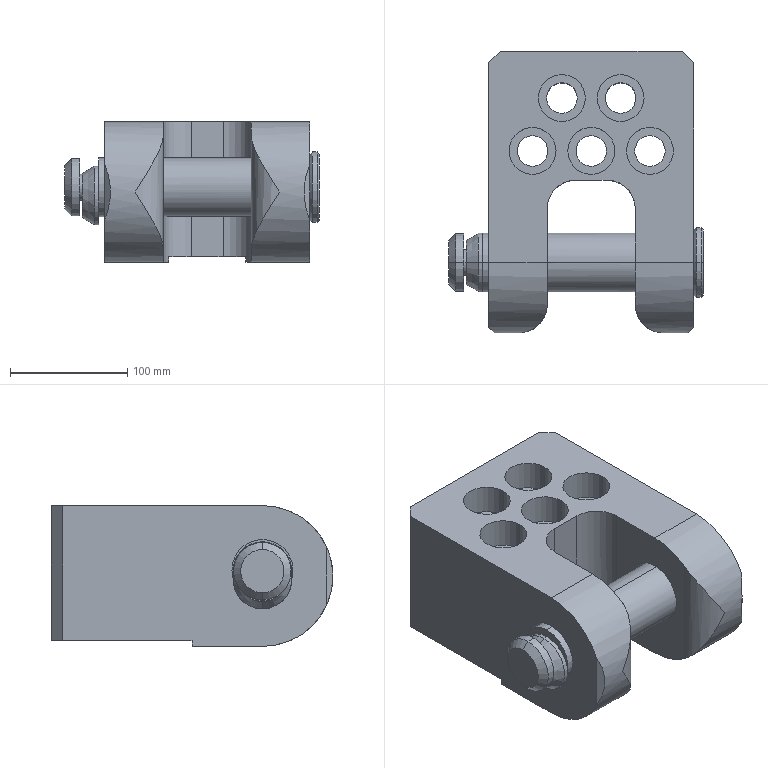Part | STEP file | 1_id4402_x_t | 1 solid | 213 faces | box 217 x 240 x 120 mm | volume 3421641 mm3 | plane 121 | cylinder 42 | other 42 | cone 8 | commonest cylinder face diameters 26 x10 40 x10 48 x4 50 x4 52 x4 22 x2